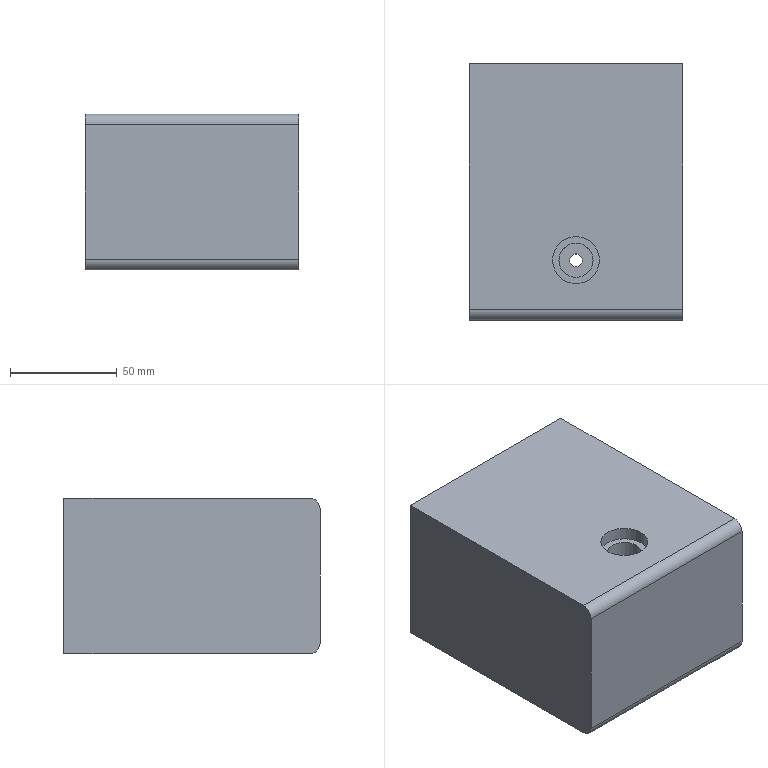Part | SolidWorks | features ICE 3, MoveFace 2, Extrusion 1, Fillet 1, HoleWzd 1 | 1 solid | 40 faces | box 100 x 120 x 73 mm | volume 861044 mm3 | cylinder 16 | cone 16 | plane 8 | commonest cylinder face diameters 8.5 x8 6 x2 10 x2 16 x2 22 x2
STEP:
#1=CARTESIAN_POINT('',(-8.,38.,6.5));
#2=VERTEX_POINT('',#1);
#3=CARTESIAN_POINT('',(8.,38.,6.5));
#4=VERTEX_POINT('',#3);
#5=CARTESIAN_POINT('',(0.,38.,6.5));
#6=DIRECTION('',(0.,0.,1.));
#7=DIRECTION('',(1.,0.,0.));
#8=AXIS2_PLACEMENT_3D('',#5,#6,#7);
#9=CIRCLE('',#8,8.);
#10=EDGE_CURVE('',#2,#4,#9,.T.);
#11=ORIENTED_EDGE('',*,*,#10,.F.);
#12=CARTESIAN_POINT('',(-8.,38.,30.5));
#13=VERTEX_POINT('',#12);
#14=CARTESIAN_POINT('',(-8.,38.,6.5));
#15=DIRECTION('',(0.,0.,1.));
#16=VECTOR('',#15,1000.);
#17=LINE('',#14,#16);
#18=EDGE_CURVE('',#2,#13,#17,.T.);
#19=ORIENTED_EDGE('',*,*,#18,.T.);
#20=CARTESIAN_POINT('',(8.,38.,30.5));
#21=VERTEX_POINT('',#20);
#22=CARTESIAN_POINT('',(0.,38.,30.5));
#23=DIRECTION('',(0.,0.,1.));
#24=DIRECTION('',(1.,0.,0.));
#25=AXIS2_PLACEMENT_3D('',#22,#23,#24);
#26=CIRCLE('',#25,8.);
#27=EDGE_CURVE('',#13,#21,#26,.T.);
#28=ORIENTED_EDGE('',*,*,#27,.T.);
#29=CARTESIAN_POINT('',(8.,38.,6.5));
#30=DIRECTION('',(0.,0.,1.));
#31=VECTOR('',#30,1000.);
#32=LINE('',#29,#31);
#33=EDGE_CURVE('',#4,#21,#32,.T.);
#34=ORIENTED_EDGE('',*,*,#33,.F.);
#35=EDGE_LOOP('',(#11,#19,#28,#34));
#36=FACE_OUTER_BOUND('',#35,.T.);
#37=CARTESIAN_POINT('',(0.,38.,6.5));
#38=DIRECTION('',(0.,0.,1.));
#39=DIRECTION('',(1.,0.,0.));
#40=AXIS2_PLACEMENT_3D('',#37,#38,#39);
#41=CYLINDRICAL_SURFACE('',#40,8.);
#42=ADVANCED_FACE('',(#36),#41,.F.);
#43=CARTESIAN_POINT('',(-11.,38.,30.5));
#44=VERTEX_POINT('',#43);
#45=CARTESIAN_POINT('',(11.,38.,30.5));
#46=VERTEX_POINT('',#45);
#47=CARTESIAN_POINT('',(0.,38.,30.5));
#48=DIRECTION('',(0.,0.,1.));
#49=DIRECTION('',(1.,0.,0.));
#50=AXIS2_PLACEMENT_3D('',#47,#48,#49);
#51=CIRCLE('',#50,11.);
#52=EDGE_CURVE('',#44,#46,#51,.T.);
#53=ORIENTED_EDGE('',*,*,#52,.F.);
#54=CARTESIAN_POINT('',(-11.,38.,36.5));
#55=VERTEX_POINT('',#54);
#56=CARTESIAN_POINT('',(-11.,38.,30.5));
#57=DIRECTION('',(0.,0.,1.));
#58=VECTOR('',#57,1000.);
#59=LINE('',#56,#58);
#60=EDGE_CURVE('',#44,#55,#59,.T.);
#61=ORIENTED_EDGE('',*,*,#60,.T.);
#62=CARTESIAN_POINT('',(11.,38.,36.5));
#63=VERTEX_POINT('',#62);
#64=CARTESIAN_POINT('',(0.,38.,36.5));
#65=DIRECTION('',(0.,0.,1.));
#66=DIRECTION('',(1.,0.,0.));
#67=AXIS2_PLACEMENT_3D('',#64,#65,#66);
#68=CIRCLE('',#67,11.);
#69=EDGE_CURVE('',#55,#63,#68,.T.);
#70=ORIENTED_EDGE('',*,*,#69,.T.);
#71=CARTESIAN_POINT('',(11.,38.,30.5));
#72=DIRECTION('',(0.,0.,1.));
#73=VECTOR('',#72,1000.);
#74=LINE('',#71,#73);
#75=EDGE_CURVE('',#46,#63,#74,.T.);
#76=ORIENTED_EDGE('',*,*,#75,.F.);
#77=EDGE_LOOP('',(#53,#61,#70,#76));
#78=FACE_OUTER_BOUND('',#77,.T.);
#79=CARTESIAN_POINT('',(0.,38.,30.5));
#80=DIRECTION('',(0.,0.,1.));
#81=DIRECTION('',(1.,0.,0.));
#82=AXIS2_PLACEMENT_3D('',#79,#80,#81);
#83=CYLINDRICAL_SURFACE('',#82,11.);
#84=ADVANCED_FACE('',(#78),#83,.F.);
#85=CARTESIAN_POINT('',(-40.,129.225,-30.75));
#86=VERTEX_POINT('',#85);
#87=CARTESIAN_POINT('',(-40.,129.225,-22.25));
#88=VERTEX_POINT('',#87);
#89=CARTESIAN_POINT('',(-40.,129.225,-26.5));
#90=DIRECTION('',(0.,1.,0.));
#91=DIRECTION('',(0.,0.,1.));
#92=AXIS2_PLACEMENT_3D('',#89,#90,#91);
#93=CIRCLE('',#92,4.25);
#94=EDGE_CURVE('',#86,#88,#93,.T.);
#95=ORIENTED_EDGE('',*,*,#94,.F.);
#96=CARTESIAN_POINT('',(-40.,130.,-31.525));
#97=VERTEX_POINT('',#96);
#98=CARTESIAN_POINT('',(-40.,130.,-31.525));
#99=DIRECTION('',(0.,0.7071,-0.7071));
#100=VECTOR('',#99,1000.);
#101=LINE('',#98,#100);
#102=EDGE_CURVE('',#86,#97,#101,.T.);
#103=ORIENTED_EDGE('',*,*,#102,.T.);
#104=CARTESIAN_POINT('',(-40.,130.,-21.475));
#105=VERTEX_POINT('',#104);
#106=CARTESIAN_POINT('',(-40.,130.,-26.5));
#107=DIRECTION('',(0.,1.,0.));
#108=DIRECTION('',(0.,0.,1.));
#109=AXIS2_PLACEMENT_3D('',#106,#107,#108);
#110=CIRCLE('',#109,5.025);
#111=EDGE_CURVE('',#97,#105,#110,.T.);
#112=ORIENTED_EDGE('',*,*,#111,.T.);
#113=CARTESIAN_POINT('',(-40.,130.,-21.475));
#114=DIRECTION('',(0.,0.7071,0.7071));
#115=VECTOR('',#114,1000.);
#116=LINE('',#113,#115);
#117=EDGE_CURVE('',#88,#105,#116,.T.);
#118=ORIENTED_EDGE('',*,*,#117,.F.);
#119=EDGE_LOOP('',(#95,#103,#112,#118));
#120=FACE_OUTER_BOUND('',#119,.T.);
#121=CARTESIAN_POINT('',(-40.,130.,-26.5));
#122=DIRECTION('',(0.,1.,0.));
#123=DIRECTION('',(0.,0.,1.));
#124=AXIS2_PLACEMENT_3D('',#121,#122,#123);
#125=CONICAL_SURFACE('',#124,5.025,0.7854);
#126=ADVANCED_FACE('',(#120),#125,.F.);
#127=CARTESIAN_POINT('',(-40.,106.5,-30.75));
#128=VERTEX_POINT('',#127);
#129=CARTESIAN_POINT('',(-40.,106.5,-22.25));
#130=VERTEX_POINT('',#129);
#131=CARTESIAN_POINT('',(-40.,106.5,-26.5));
#132=DIRECTION('',(0.,1.,0.));
#133=DIRECTION('',(0.,0.,1.));
#134=AXIS2_PLACEMENT_3D('',#131,#132,#133);
#135=CIRCLE('',#134,4.25);
#136=EDGE_CURVE('',#128,#130,#135,.T.);
#137=ORIENTED_EDGE('',*,*,#136,.F.);
#138=CARTESIAN_POINT('',(-40.,130.,-30.75));
#139=DIRECTION('',(0.,1.,0.));
#140=VECTOR('',#139,1000.);
#141=LINE('',#138,#140);
#142=EDGE_CURVE('',#128,#86,#141,.T.);
#143=ORIENTED_EDGE('',*,*,#142,.T.);
#144=ORIENTED_EDGE('',*,*,#94,.T.);
#145=CARTESIAN_POINT('',(-40.,130.,-22.25));
#146=DIRECTION('',(0.,1.,0.));
#147=VECTOR('',#146,1000.);
#148=LINE('',#145,#147);
#149=EDGE_CURVE('',#130,#88,#148,.T.);
#150=ORIENTED_EDGE('',*,*,#149,.F.);
#151=EDGE_LOOP('',(#137,#143,#144,#150));
#152=FACE_OUTER_BOUND('',#151,.T.);
#153=CARTESIAN_POINT('',(-40.,130.,-26.5));
#154=DIRECTION('',(0.,1.,0.));
#155=DIRECTION('',(0.,0.,1.));
#156=AXIS2_PLACEMENT_3D('',#153,#154,#155);
#157=CYLINDRICAL_SURFACE('',#156,4.25);
#158=ADVANCED_FACE('',(#152),#157,.F.);
#159=CARTESIAN_POINT('',(-40.,103.946,-26.5));
#160=VERTEX_POINT('',#159);
#161=CARTESIAN_POINT('',(-40.,106.5,-22.25));
#162=DIRECTION('',(0.,0.515,0.8572));
#163=VECTOR('',#162,1000.);
#164=LINE('',#161,#163);
#165=EDGE_CURVE('',#160,#130,#164,.T.);
#166=ORIENTED_EDGE('',*,*,#165,.F.);
#167=CARTESIAN_POINT('',(-40.,106.5,-30.75));
#168=DIRECTION('',(0.,0.515,-0.8572));
#169=VECTOR('',#168,1000.);
#170=LINE('',#167,#169);
#171=EDGE_CURVE('',#160,#128,#170,.T.);
#172=ORIENTED_EDGE('',*,*,#171,.T.);
#173=ORIENTED_EDGE('',*,*,#136,.T.);
#174=EDGE_LOOP('',(#166,#172,#173));
#175=FACE_OUTER_BOUND('',#174,.T.);
#176=CARTESIAN_POINT('',(-40.,106.5,-26.5));
#177=DIRECTION('',(0.,1.,0.));
#178=DIRECTION('',(0.,0.,1.));
#179=AXIS2_PLACEMENT_3D('',#176,#177,#178);
#180=CONICAL_SURFACE('',#179,4.25,1.03);
#181=ADVANCED_FACE('',(#175),#180,.F.);
#182=CARTESIAN_POINT('',(40.,129.225,-30.75));
#183=VERTEX_POINT('',#182);
#184=CARTESIAN_POINT('',(40.,129.225,-22.25));
#185=VERTEX_POINT('',#184);
#186=CARTESIAN_POINT('',(40.,129.225,-26.5));
#187=DIRECTION('',(0.,1.,0.));
#188=DIRECTION('',(0.,0.,1.));
#189=AXIS2_PLACEMENT_3D('',#186,#187,#188);
#190=CIRCLE('',#189,4.25);
#191=EDGE_CURVE('',#183,#185,#190,.T.);
#192=ORIENTED_EDGE('',*,*,#191,.F.);
#193=CARTESIAN_POINT('',(40.,130.,-31.525));
#194=VERTEX_POINT('',#193);
#195=CARTESIAN_POINT('',(40.,130.,-31.525));
#196=DIRECTION('',(0.,0.7071,-0.7071));
#197=VECTOR('',#196,1000.);
#198=LINE('',#195,#197);
#199=EDGE_CURVE('',#183,#194,#198,.T.);
#200=ORIENTED_EDGE('',*,*,#199,.T.);
#201=CARTESIAN_POINT('',(40.,130.,-21.475));
#202=VERTEX_POINT('',#201);
#203=CARTESIAN_POINT('',(40.,130.,-26.5));
#204=DIRECTION('',(0.,1.,0.));
#205=DIRECTION('',(0.,0.,1.));
#206=AXIS2_PLACEMENT_3D('',#203,#204,#205);
#207=CIRCLE('',#206,5.025);
#208=EDGE_CURVE('',#194,#202,#207,.T.);
#209=ORIENTED_EDGE('',*,*,#208,.T.);
#210=CARTESIAN_POINT('',(40.,130.,-21.475));
#211=DIRECTION('',(0.,0.7071,0.7071));
#212=VECTOR('',#211,1000.);
#213=LINE('',#210,#212);
#214=EDGE_CURVE('',#185,#202,#213,.T.);
#215=ORIENTED_EDGE('',*,*,#214,.F.);
#216=EDGE_LOOP('',(#192,#200,#209,#215));
#217=FACE_OUTER_BOUND('',#216,.T.);
#218=CARTESIAN_POINT('',(40.,130.,-26.5));
#219=DIRECTION('',(0.,1.,0.));
#220=DIRECTION('',(0.,0.,1.));
#221=AXIS2_PLACEMENT_3D('',#218,#219,#220);
#222=CONICAL_SURFACE('',#221,5.025,0.7854);
#223=ADVANCED_FACE('',(#217),#222,.F.);
#224=CARTESIAN_POINT('',(40.,106.5,-30.75));
#225=VERTEX_POINT('',#224);
#226=CARTESIAN_POINT('',(40.,106.5,-22.25));
#227=VERTEX_POINT('',#226);
#228=CARTESIAN_POINT('',(40.,106.5,-26.5));
#229=DIRECTION('',(0.,1.,0.));
#230=DIRECTION('',(0.,0.,1.));
#231=AXIS2_PLACEMENT_3D('',#228,#229,#230);
#232=CIRCLE('',#231,4.25);
#233=EDGE_CURVE('',#225,#227,#232,.T.);
#234=ORIENTED_EDGE('',*,*,#233,.F.);
#235=CARTESIAN_POINT('',(40.,130.,-30.75));
#236=DIRECTION('',(0.,1.,0.));
#237=VECTOR('',#236,1000.);
#238=LINE('',#235,#237);
#239=EDGE_CURVE('',#225,#183,#238,.T.);
#240=ORIENTED_EDGE('',*,*,#239,.T.);
#241=ORIENTED_EDGE('',*,*,#191,.T.);
#242=CARTESIAN_POINT('',(40.,130.,-22.25));
#243=DIRECTION('',(0.,1.,0.));
#244=VECTOR('',#243,1000.);
#245=LINE('',#242,#244);
#246=EDGE_CURVE('',#227,#185,#245,.T.);
#247=ORIENTED_EDGE('',*,*,#246,.F.);
#248=EDGE_LOOP('',(#234,#240,#241,#247));
#249=FACE_OUTER_BOUND('',#248,.T.);
#250=CARTESIAN_POINT('',(40.,130.,-26.5));
#251=DIRECTION('',(0.,1.,0.));
#252=DIRECTION('',(0.,0.,1.));
#253=AXIS2_PLACEMENT_3D('',#250,#251,#252);
#254=CYLINDRICAL_SURFACE('',#253,4.25);
#255=ADVANCED_FACE('',(#249),#254,.F.);
#256=CARTESIAN_POINT('',(40.,103.946,-26.5));
#257=VERTEX_POINT('',#256);
#258=CARTESIAN_POINT('',(40.,106.5,-22.25));
#259=DIRECTION('',(0.,0.515,0.8572));
#260=VECTOR('',#259,1000.);
#261=LINE('',#258,#260);
#262=EDGE_CURVE('',#257,#227,#261,.T.);
#263=ORIENTED_EDGE('',*,*,#262,.F.);
#264=CARTESIAN_POINT('',(40.,106.5,-30.75));
#265=DIRECTION('',(0.,0.515,-0.8572));
#266=VECTOR('',#265,1000.);
#267=LINE('',#264,#266);
#268=EDGE_CURVE('',#257,#225,#267,.T.);
#269=ORIENTED_EDGE('',*,*,#268,.T.);
#270=ORIENTED_EDGE('',*,*,#233,.T.);
#271=EDGE_LOOP('',(#263,#269,#270));
#272=FACE_OUTER_BOUND('',#271,.T.);
#273=CARTESIAN_POINT('',(40.,106.5,-26.5));
#274=DIRECTION('',(0.,1.,0.));
#275=DIRECTION('',(0.,0.,1.));
#276=AXIS2_PLACEMENT_3D('',#273,#274,#275);
#277=CONICAL_SURFACE('',#276,4.25,1.03);
#278=ADVANCED_FACE('',(#272),#277,.F.);
#279=CARTESIAN_POINT('',(40.,129.225,2.25));
#280=VERTEX_POINT('',#279);
#281=CARTESIAN_POINT('',(40.,129.225,10.75));
#282=VERTEX_POINT('',#281);
#283=CARTESIAN_POINT('',(40.,129.225,6.5));
#284=DIRECTION('',(0.,1.,0.));
#285=DIRECTION('',(0.,0.,1.));
#286=AXIS2_PLACEMENT_3D('',#283,#284,#285);
#287=CIRCLE('',#286,4.25);
#288=EDGE_CURVE('',#280,#282,#287,.T.);
#289=ORIENTED_EDGE('',*,*,#288,.F.);
#290=CARTESIAN_POINT('',(40.,130.,1.475));
#291=VERTEX_POINT('',#290);
#292=CARTESIAN_POINT('',(40.,130.,1.475));
#293=DIRECTION('',(0.,0.7071,-0.7071));
#294=VECTOR('',#293,1000.);
#295=LINE('',#292,#294);
#296=EDGE_CURVE('',#280,#291,#295,.T.);
#297=ORIENTED_EDGE('',*,*,#296,.T.);
#298=CARTESIAN_POINT('',(40.,130.,11.525));
#299=VERTEX_POINT('',#298);
#300=CARTESIAN_POINT('',(40.,130.,6.5));
#301=DIRECTION('',(0.,1.,0.));
#302=DIRECTION('',(0.,0.,1.));
#303=AXIS2_PLACEMENT_3D('',#300,#301,#302);
#304=CIRCLE('',#303,5.025);
#305=EDGE_CURVE('',#291,#299,#304,.T.);
#306=ORIENTED_EDGE('',*,*,#305,.T.);
#307=CARTESIAN_POINT('',(40.,130.,11.525));
#308=DIRECTION('',(0.,0.7071,0.7071));
#309=VECTOR('',#308,1000.);
#310=LINE('',#307,#309);
#311=EDGE_CURVE('',#282,#299,#310,.T.);
#312=ORIENTED_EDGE('',*,*,#311,.F.);
#313=EDGE_LOOP('',(#289,#297,#306,#312));
#314=FACE_OUTER_BOUND('',#313,.T.);
#315=CARTESIAN_POINT('',(40.,130.,6.5));
#316=DIRECTION('',(0.,1.,0.));
#317=DIRECTION('',(0.,0.,1.));
#318=AXIS2_PLACEMENT_3D('',#315,#316,#317);
#319=CONICAL_SURFACE('',#318,5.025,0.7854);
#320=ADVANCED_FACE('',(#314),#319,.F.);
#321=CARTESIAN_POINT('',(40.,106.5,2.25));
#322=VERTEX_POINT('',#321);
#323=CARTESIAN_POINT('',(40.,106.5,10.75));
#324=VERTEX_POINT('',#323);
#325=CARTESIAN_POINT('',(40.,106.5,6.5));
#326=DIRECTION('',(0.,1.,0.));
#327=DIRECTION('',(0.,0.,1.));
#328=AXIS2_PLACEMENT_3D('',#325,#326,#327);
#329=CIRCLE('',#328,4.25);
#330=EDGE_CURVE('',#322,#324,#329,.T.);
#331=ORIENTED_EDGE('',*,*,#330,.F.);
#332=CARTESIAN_POINT('',(40.,130.,2.25));
#333=DIRECTION('',(0.,1.,0.));
#334=VECTOR('',#333,1000.);
#335=LINE('',#332,#334);
#336=EDGE_CURVE('',#322,#280,#335,.T.);
#337=ORIENTED_EDGE('',*,*,#336,.T.);
#338=ORIENTED_EDGE('',*,*,#288,.T.);
#339=CARTESIAN_POINT('',(40.,130.,10.75));
#340=DIRECTION('',(0.,1.,0.));
#341=VECTOR('',#340,1000.);
#342=LINE('',#339,#341);
#343=EDGE_CURVE('',#324,#282,#342,.T.);
#344=ORIENTED_EDGE('',*,*,#343,.F.);
#345=EDGE_LOOP('',(#331,#337,#338,#344));
#346=FACE_OUTER_BOUND('',#345,.T.);
#347=CARTESIAN_POINT('',(40.,130.,6.5));
#348=DIRECTION('',(0.,1.,0.));
#349=DIRECTION('',(0.,0.,1.));
#350=AXIS2_PLACEMENT_3D('',#347,#348,#349);
#351=CYLINDRICAL_SURFACE('',#350,4.25);
#352=ADVANCED_FACE('',(#346),#351,.F.);
#353=CARTESIAN_POINT('',(40.,103.946,6.5));
#354=VERTEX_POINT('',#353);
#355=CARTESIAN_POINT('',(40.,106.5,10.75));
#356=DIRECTION('',(0.,0.515,0.8572));
#357=VECTOR('',#356,1000.);
#358=LINE('',#355,#357);
#359=EDGE_CURVE('',#354,#324,#358,.T.);
#360=ORIENTED_EDGE('',*,*,#359,.F.);
#361=CARTESIAN_POINT('',(40.,106.5,2.25));
#362=DIRECTION('',(0.,0.515,-0.8572));
#363=VECTOR('',#362,1000.);
#364=LINE('',#361,#363);
#365=EDGE_CURVE('',#354,#322,#364,.T.);
#366=ORIENTED_EDGE('',*,*,#365,.T.);
#367=ORIENTED_EDGE('',*,*,#330,.T.);
#368=EDGE_LOOP('',(#360,#366,#367));
#369=FACE_OUTER_BOUND('',#368,.T.);
#370=CARTESIAN_POINT('',(40.,106.5,6.5));
#371=DIRECTION('',(0.,1.,0.));
#372=DIRECTION('',(0.,0.,1.));
#373=AXIS2_PLACEMENT_3D('',#370,#371,#372);
#374=CONICAL_SURFACE('',#373,4.25,1.03);
#375=ADVANCED_FACE('',(#369),#374,.F.);
#376=CARTESIAN_POINT('',(-40.,129.225,2.25));
#377=VERTEX_POINT('',#376);
#378=CARTESIAN_POINT('',(-40.,129.225,10.75));
#379=VERTEX_POINT('',#378);
#380=CARTESIAN_POINT('',(-40.,129.225,6.5));
#381=DIRECTION('',(0.,1.,0.));
#382=DIRECTION('',(0.,0.,1.));
#383=AXIS2_PLACEMENT_3D('',#380,#381,#382);
#384=CIRCLE('',#383,4.25);
#385=EDGE_CURVE('',#377,#379,#384,.T.);
#386=ORIENTED_EDGE('',*,*,#385,.F.);
#387=CARTESIAN_POINT('',(-40.,130.,1.475));
#388=VERTEX_POINT('',#387);
#389=CARTESIAN_POINT('',(-40.,130.,1.475));
#390=DIRECTION('',(0.,0.7071,-0.7071));
#391=VECTOR('',#390,1000.);
#392=LINE('',#389,#391);
#393=EDGE_CURVE('',#377,#388,#392,.T.);
#394=ORIENTED_EDGE('',*,*,#393,.T.);
#395=CARTESIAN_POINT('',(-40.,130.,11.525));
#396=VERTEX_POINT('',#395);
#397=CARTESIAN_POINT('',(-40.,130.,6.5));
#398=DIRECTION('',(0.,1.,0.));
#399=DIRECTION('',(0.,0.,1.));
#400=AXIS2_PLACEMENT_3D('',#397,#398,#399);
#401=CIRCLE('',#400,5.025);
#402=EDGE_CURVE('',#388,#396,#401,.T.);
#403=ORIENTED_EDGE('',*,*,#402,.T.);
#404=CARTESIAN_POINT('',(-40.,130.,11.525));
#405=DIRECTION('',(0.,0.7071,0.7071));
#406=VECTOR('',#405,1000.);
#407=LINE('',#404,#406);
#408=EDGE_CURVE('',#379,#396,#407,.T.);
#409=ORIENTED_EDGE('',*,*,#408,.F.);
#410=EDGE_LOOP('',(#386,#394,#403,#409));
#411=FACE_OUTER_BOUND('',#410,.T.);
#412=CARTESIAN_POINT('',(-40.,130.,6.5));
#413=DIRECTION('',(0.,1.,0.));
#414=DIRECTION('',(0.,0.,1.));
#415=AXIS2_PLACEMENT_3D('',#412,#413,#414);
#416=CONICAL_SURFACE('',#415,5.025,0.7854);
#417=ADVANCED_FACE('',(#411),#416,.F.);
#418=CARTESIAN_POINT('',(-40.,106.5,2.25));
#419=VERTEX_POINT('',#418);
#420=CARTESIAN_POINT('',(-40.,106.5,10.75));
#421=VERTEX_POINT('',#420);
#422=CARTESIAN_POINT('',(-40.,106.5,6.5));
#423=DIRECTION('',(0.,1.,0.));
#424=DIRECTION('',(0.,0.,1.));
#425=AXIS2_PLACEMENT_3D('',#422,#423,#424);
#426=CIRCLE('',#425,4.25);
#427=EDGE_CURVE('',#419,#421,#426,.T.);
#428=ORIENTED_EDGE('',*,*,#427,.F.);
#429=CARTESIAN_POINT('',(-40.,130.,2.25));
#430=DIRECTION('',(0.,1.,0.));
#431=VECTOR('',#430,1000.);
#432=LINE('',#429,#431);
#433=EDGE_CURVE('',#419,#377,#432,.T.);
#434=ORIENTED_EDGE('',*,*,#433,.T.);
#435=ORIENTED_EDGE('',*,*,#385,.T.);
#436=CARTESIAN_POINT('',(-40.,130.,10.75));
#437=DIRECTION('',(0.,1.,0.));
#438=VECTOR('',#437,1000.);
#439=LINE('',#436,#438);
#440=EDGE_CURVE('',#421,#379,#439,.T.);
#441=ORIENTED_EDGE('',*,*,#440,.F.);
#442=EDGE_LOOP('',(#428,#434,#435,#441));
#443=FACE_OUTER_BOUND('',#442,.T.);
#444=CARTESIAN_POINT('',(-40.,130.,6.5));
#445=DIRECTION('',(0.,1.,0.));
#446=DIRECTION('',(0.,0.,1.));
#447=AXIS2_PLACEMENT_3D('',#444,#445,#446);
#448=CYLINDRICAL_SURFACE('',#447,4.25);
#449=ADVANCED_FACE('',(#443),#448,.F.);
#450=CARTESIAN_POINT('',(-40.,103.946,6.5));
#451=VERTEX_POINT('',#450);
#452=CARTESIAN_POINT('',(-40.,106.5,10.75));
#453=DIRECTION('',(0.,0.515,0.8572));
#454=VECTOR('',#453,1000.);
#455=LINE('',#452,#454);
#456=EDGE_CURVE('',#451,#421,#455,.T.);
#457=ORIENTED_EDGE('',*,*,#456,.F.);
#458=CARTESIAN_POINT('',(-40.,106.5,2.25));
#459=DIRECTION('',(0.,0.515,-0.8572));
#460=VECTOR('',#459,1000.);
#461=LINE('',#458,#460);
#462=EDGE_CURVE('',#451,#419,#461,.T.);
#463=ORIENTED_EDGE('',*,*,#462,.T.);
#464=ORIENTED_EDGE('',*,*,#427,.T.);
#465=EDGE_LOOP('',(#457,#463,#464));
#466=FACE_OUTER_BOUND('',#465,.T.);
#467=CARTESIAN_POINT('',(-40.,106.5,6.5));
#468=DIRECTION('',(0.,1.,0.));
#469=DIRECTION('',(0.,0.,1.));
#470=AXIS2_PLACEMENT_3D('',#467,#468,#469);
#471=CONICAL_SURFACE('',#470,4.25,1.03);
#472=ADVANCED_FACE('',(#466),#471,.F.);
#473=CARTESIAN_POINT('',(3.,38.,6.5));
#474=VERTEX_POINT('',#473);
#475=CARTESIAN_POINT('',(-3.,38.,6.5));
#476=VERTEX_POINT('',#475);
#477=CARTESIAN_POINT('',(0.,38.,6.5));
#478=DIRECTION('',(0.,0.,-1.));
#479=DIRECTION('',(1.,0.,0.));
#480=AXIS2_PLACEMENT_3D('',#477,#478,#479);
#481=CIRCLE('',#480,3.);
#482=EDGE_CURVE('',#474,#476,#481,.T.);
#483=ORIENTED_EDGE('',*,*,#482,.F.);
#484=CARTESIAN_POINT('',(3.,38.,-36.5));
#485=VERTEX_POINT('',#484);
#486=CARTESIAN_POINT('',(3.,38.,93.5));
#487=DIRECTION('',(0.,0.,-1.));
#488=VECTOR('',#487,1000.);
#489=LINE('',#486,#488);
#490=EDGE_CURVE('',#474,#485,#489,.T.);
#491=ORIENTED_EDGE('',*,*,#490,.T.);
#492=CARTESIAN_POINT('',(-3.,38.,-36.5));
#493=VERTEX_POINT('',#492);
#494=CARTESIAN_POINT('',(0.,38.,-36.5));
#495=DIRECTION('',(0.,0.,-1.));
#496=DIRECTION('',(-1.,0.,0.));
#497=AXIS2_PLACEMENT_3D('',#494,#495,#496);
#498=CIRCLE('',#497,3.);
#499=EDGE_CURVE('',#485,#493,#498,.T.);
#500=ORIENTED_EDGE('',*,*,#499,.T.);
#501=CARTESIAN_POINT('',(-3.,38.,93.5));
#502=DIRECTION('',(0.,0.,-1.));
#503=VECTOR('',#502,1000.);
#504=LINE('',#501,#503);
#505=EDGE_CURVE('',#476,#493,#504,.T.);
#506=ORIENTED_EDGE('',*,*,#505,.F.);
#507=EDGE_LOOP('',(#483,#491,#500,#506));
#508=FACE_OUTER_BOUND('',#507,.T.);
#509=CARTESIAN_POINT('',(0.,38.,93.5));
#510=DIRECTION('',(0.,0.,-1.));
#511=DIRECTION('',(-1.,0.,0.));
#512=AXIS2_PLACEMENT_3D('',#509,#510,#511);
#513=CYLINDRICAL_SURFACE('',#512,3.);
#514=ADVANCED_FACE('',(#508),#513,.F.);
#515=ORIENTED_EDGE('',*,*,#490,.F.);
#516=CARTESIAN_POINT('',(0.,38.,6.5));
#517=DIRECTION('',(0.,0.,-1.));
#518=DIRECTION('',(1.,0.,0.));
#519=AXIS2_PLACEMENT_3D('',#516,#517,#518);
#520=CIRCLE('',#519,3.);
#521=EDGE_CURVE('',#476,#474,#520,.T.);
#522=ORIENTED_EDGE('',*,*,#521,.F.);
#523=ORIENTED_EDGE('',*,*,#505,.T.);
#524=CARTESIAN_POINT('',(0.,38.,-36.5));
#525=DIRECTION('',(0.,0.,-1.));
#526=DIRECTION('',(-1.,0.,0.));
#527=AXIS2_PLACEMENT_3D('',#524,#525,#526);
#528=CIRCLE('',#527,3.);
#529=EDGE_CURVE('',#493,#485,#528,.T.);
#530=ORIENTED_EDGE('',*,*,#529,.T.);
#531=EDGE_LOOP('',(#515,#522,#523,#530));
#532=FACE_OUTER_BOUND('',#531,.T.);
#533=CARTESIAN_POINT('',(0.,38.,93.5));
#534=DIRECTION('',(0.,0.,-1.));
#535=DIRECTION('',(-1.,0.,0.));
#536=AXIS2_PLACEMENT_3D('',#533,#534,#535);
#537=CYLINDRICAL_SURFACE('',#536,3.);
#538=ADVANCED_FACE('',(#532),#537,.F.);
#539=CARTESIAN_POINT('',(50.,10.,31.5));
#540=VERTEX_POINT('',#539);
#541=CARTESIAN_POINT('',(50.,10.,-31.5));
#542=VERTEX_POINT('',#541);
#543=CARTESIAN_POINT('',(50.,10.,36.5));
#544=DIRECTION('',(0.,0.,-1.));
#545=VECTOR('',#544,1000.);
#546=LINE('',#543,#545);
#547=EDGE_CURVE('',#540,#542,#546,.T.);
#548=ORIENTED_EDGE('',*,*,#547,.T.);
#549=CARTESIAN_POINT('',(50.,15.,-36.5));
#550=VERTEX_POINT('',#549);
#551=CARTESIAN_POINT('',(50.,15.,-31.5));
#552=DIRECTION('',(1.,0.,0.));
#553=DIRECTION('',(0.,0.,1.));
#554=AXIS2_PLACEMENT_3D('',#551,#552,#553);
#555=CIRCLE('',#554,5.);
#556=EDGE_CURVE('',#542,#550,#555,.T.);
#557=ORIENTED_EDGE('',*,*,#556,.T.);
#558=CARTESIAN_POINT('',(50.,130.,-36.5));
#559=VERTEX_POINT('',#558);
#560=CARTESIAN_POINT('',(50.,130.,-36.5));
#561=DIRECTION('',(0.,-1.,0.));
#562=VECTOR('',#561,1000.);
#563=LINE('',#560,#562);
#564=EDGE_CURVE('',#559,#550,#563,.T.);
#565=ORIENTED_EDGE('',*,*,#564,.F.);
#566=CARTESIAN_POINT('',(50.,130.,36.5));
#567=VERTEX_POINT('',#566);
#568=CARTESIAN_POINT('',(50.,130.,36.5));
#569=DIRECTION('',(0.,0.,-1.));
#570=VECTOR('',#569,1000.);
#571=LINE('',#568,#570);
#572=EDGE_CURVE('',#567,#559,#571,.T.);
#573=ORIENTED_EDGE('',*,*,#572,.F.);
#574=CARTESIAN_POINT('',(50.,15.,36.5));
#575=VERTEX_POINT('',#574);
#576=CARTESIAN_POINT('',(50.,130.,36.5));
#577=DIRECTION('',(0.,-1.,0.));
#578=VECTOR('',#577,1000.);
#579=LINE('',#576,#578);
#580=EDGE_CURVE('',#567,#575,#579,.T.);
#581=ORIENTED_EDGE('',*,*,#580,.T.);
#582=CARTESIAN_POINT('',(50.,15.,31.5));
#583=DIRECTION('',(1.,0.,0.));
#584=DIRECTION('',(0.,0.,1.));
#585=AXIS2_PLACEMENT_3D('',#582,#583,#584);
#586=CIRCLE('',#585,5.);
#587=EDGE_CURVE('',#575,#540,#586,.T.);
#588=ORIENTED_EDGE('',*,*,#587,.T.);
#589=EDGE_LOOP('',(#548,#557,#565,#573,#581,#588));
#590=FACE_OUTER_BOUND('',#589,.T.);
#591=CARTESIAN_POINT('',(50.,130.,36.5));
#592=DIRECTION('',(-1.,0.,0.));
#593=DIRECTION('',(0.,0.,1.));
#594=AXIS2_PLACEMENT_3D('',#591,#592,#593);
#595=PLANE('',#594);
#596=ADVANCED_FACE('',(#590),#595,.F.);
#597=ORIENTED_EDGE('',*,*,#529,.F.);
#598=ORIENTED_EDGE('',*,*,#499,.F.);
#599=EDGE_LOOP('',(#597,#598));
#600=FACE_BOUND('',#599,.T.);
#601=ORIENTED_EDGE('',*,*,#564,.T.);
#602=CARTESIAN_POINT('',(-50.,15.,-36.5));
#603=VERTEX_POINT('',#602);
#604=CARTESIAN_POINT('',(-50.,15.,-36.5));
#605=DIRECTION('',(-1.,0.,0.));
#606=VECTOR('',#605,1000.);
#607=LINE('',#604,#606);
#608=EDGE_CURVE('',#550,#603,#607,.T.);
#609=ORIENTED_EDGE('',*,*,#608,.T.);
#610=CARTESIAN_POINT('',(-50.,130.,-36.5));
#611=VERTEX_POINT('',#610);
#612=CARTESIAN_POINT('',(-50.,130.,-36.5));
#613=DIRECTION('',(0.,-1.,0.));
#614=VECTOR('',#613,1000.);
#615=LINE('',#612,#614);
#616=EDGE_CURVE('',#611,#603,#615,.T.);
#617=ORIENTED_EDGE('',*,*,#616,.F.);
#618=CARTESIAN_POINT('',(-50.,130.,-36.5));
#619=DIRECTION('',(-1.,0.,0.));
#620=VECTOR('',#619,1000.);
#621=LINE('',#618,#620);
#622=EDGE_CURVE('',#559,#611,#621,.T.);
#623=ORIENTED_EDGE('',*,*,#622,.F.);
#624=EDGE_LOOP('',(#601,#609,#617,#623));
#625=FACE_OUTER_BOUND('',#624,.T.);
#626=CARTESIAN_POINT('',(-50.,130.,-36.5));
#627=DIRECTION('',(0.,0.,1.));
#628=DIRECTION('',(1.,0.,0.));
#629=AXIS2_PLACEMENT_3D('',#626,#627,#628);
#630=PLANE('',#629);
#631=ADVANCED_FACE('',(#600,#625),#630,.F.);
#632=ORIENTED_EDGE('',*,*,#616,.T.);
#633=CARTESIAN_POINT('',(-50.,10.,-31.5));
#634=VERTEX_POINT('',#633);
#635=CARTESIAN_POINT('',(-50.,15.,-31.5));
#636=DIRECTION('',(-1.,0.,0.));
#637=DIRECTION('',(0.,0.,-1.));
#638=AXIS2_PLACEMENT_3D('',#635,#636,#637);
#639=CIRCLE('',#638,5.);
#640=EDGE_CURVE('',#603,#634,#639,.T.);
#641=ORIENTED_EDGE('',*,*,#640,.T.);
#642=CARTESIAN_POINT('',(-50.,10.,31.5));
#643=VERTEX_POINT('',#642);
#644=CARTESIAN_POINT('',(-50.,10.,36.5));
#645=DIRECTION('',(0.,0.,1.));
#646=VECTOR('',#645,1000.);
#647=LINE('',#644,#646);
#648=EDGE_CURVE('',#634,#643,#647,.T.);
#649=ORIENTED_EDGE('',*,*,#648,.T.);
#650=CARTESIAN_POINT('',(-50.,15.,36.5));
#651=VERTEX_POINT('',#650);
#652=CARTESIAN_POINT('',(-50.,15.,31.5));
#653=DIRECTION('',(-1.,0.,0.));
#654=DIRECTION('',(0.,0.,-1.));
#655=AXIS2_PLACEMENT_3D('',#652,#653,#654);
#656=CIRCLE('',#655,5.);
#657=EDGE_CURVE('',#643,#651,#656,.T.);
#658=ORIENTED_EDGE('',*,*,#657,.T.);
#659=CARTESIAN_POINT('',(-50.,130.,36.5));
#660=VERTEX_POINT('',#659);
#661=CARTESIAN_POINT('',(-50.,130.,36.5));
#662=DIRECTION('',(0.,-1.,0.));
#663=VECTOR('',#662,1000.);
#664=LINE('',#661,#663);
#665=EDGE_CURVE('',#660,#651,#664,.T.);
#666=ORIENTED_EDGE('',*,*,#665,.F.);
#667=CARTESIAN_POINT('',(-50.,130.,36.5));
#668=DIRECTION('',(0.,0.,1.));
#669=VECTOR('',#668,1000.);
#670=LINE('',#667,#669);
#671=EDGE_CURVE('',#611,#660,#670,.T.);
#672=ORIENTED_EDGE('',*,*,#671,.F.);
#673=EDGE_LOOP('',(#632,#641,#649,#658,#666,#672));
#674=FACE_OUTER_BOUND('',#673,.T.);
#675=CARTESIAN_POINT('',(-50.,130.,36.5));
#676=DIRECTION('',(1.,0.,0.));
#677=DIRECTION('',(0.,0.,-1.));
#678=AXIS2_PLACEMENT_3D('',#675,#676,#677);
#679=PLANE('',#678);
#680=ADVANCED_FACE('',(#674),#679,.F.);
#681=CARTESIAN_POINT('',(0.,38.,36.5));
#682=DIRECTION('',(0.,0.,1.));
#683=DIRECTION('',(1.,0.,0.));
#684=AXIS2_PLACEMENT_3D('',#681,#682,#683);
#685=CIRCLE('',#684,11.);
#686=EDGE_CURVE('',#63,#55,#685,.T.);
#687=ORIENTED_EDGE('',*,*,#686,.F.);
#688=ORIENTED_EDGE('',*,*,#69,.F.);
#689=EDGE_LOOP('',(#687,#688));
#690=FACE_BOUND('',#689,.T.);
#691=ORIENTED_EDGE('',*,*,#665,.T.);
#692=CARTESIAN_POINT('',(50.,15.,36.5));
#693=DIRECTION('',(1.,0.,0.));
#694=VECTOR('',#693,1000.);
#695=LINE('',#692,#694);
#696=EDGE_CURVE('',#651,#575,#695,.T.);
#697=ORIENTED_EDGE('',*,*,#696,.T.);
#698=ORIENTED_EDGE('',*,*,#580,.F.);
#699=CARTESIAN_POINT('',(-50.,130.,36.5));
#700=DIRECTION('',(1.,0.,0.));
#701=VECTOR('',#700,1000.);
#702=LINE('',#699,#701);
#703=EDGE_CURVE('',#660,#567,#702,.T.);
#704=ORIENTED_EDGE('',*,*,#703,.F.);
#705=EDGE_LOOP('',(#691,#697,#698,#704));
#706=FACE_OUTER_BOUND('',#705,.T.);
#707=CARTESIAN_POINT('',(-50.,130.,36.5));
#708=DIRECTION('',(0.,0.,-1.));
#709=DIRECTION('',(-1.,0.,0.));
#710=AXIS2_PLACEMENT_3D('',#707,#708,#709);
#711=PLANE('',#710);
#712=ADVANCED_FACE('',(#690,#706),#711,.F.);
#713=CARTESIAN_POINT('',(-40.,130.,-26.5));
#714=DIRECTION('',(0.,1.,0.));
#715=DIRECTION('',(0.,0.,1.));
#716=AXIS2_PLACEMENT_3D('',#713,#714,#715);
#717=CIRCLE('',#716,5.025);
#718=EDGE_CURVE('',#105,#97,#717,.T.);
#719=ORIENTED_EDGE('',*,*,#718,.F.);
#720=ORIENTED_EDGE('',*,*,#111,.F.);
#721=EDGE_LOOP('',(#719,#720));
#722=FACE_BOUND('',#721,.T.);
#723=CARTESIAN_POINT('',(40.,130.,-26.5));
#724=DIRECTION('',(0.,1.,0.));
#725=DIRECTION('',(0.,0.,1.));
#726=AXIS2_PLACEMENT_3D('',#723,#724,#725);
#727=CIRCLE('',#726,5.025);
#728=EDGE_CURVE('',#202,#194,#727,.T.);
#729=ORIENTED_EDGE('',*,*,#728,.F.);
#730=ORIENTED_EDGE('',*,*,#208,.F.);
#731=EDGE_LOOP('',(#729,#730));
#732=FACE_BOUND('',#731,.T.);
#733=CARTESIAN_POINT('',(40.,130.,6.5));
#734=DIRECTION('',(0.,1.,0.));
#735=DIRECTION('',(0.,0.,1.));
#736=AXIS2_PLACEMENT_3D('',#733,#734,#735);
#737=CIRCLE('',#736,5.025);
#738=EDGE_CURVE('',#299,#291,#737,.T.);
#739=ORIENTED_EDGE('',*,*,#738,.F.);
#740=ORIENTED_EDGE('',*,*,#305,.F.);
#741=EDGE_LOOP('',(#739,#740));
#742=FACE_BOUND('',#741,.T.);
#743=CARTESIAN_POINT('',(-40.,130.,6.5));
#744=DIRECTION('',(0.,1.,0.));
#745=DIRECTION('',(0.,0.,1.));
#746=AXIS2_PLACEMENT_3D('',#743,#744,#745);
#747=CIRCLE('',#746,5.025);
#748=EDGE_CURVE('',#396,#388,#747,.T.);
#749=ORIENTED_EDGE('',*,*,#748,.F.);
#750=ORIENTED_EDGE('',*,*,#402,.F.);
#751=EDGE_LOOP('',(#749,#750));
#752=FACE_BOUND('',#751,.T.);
#753=ORIENTED_EDGE('',*,*,#572,.T.);
#754=ORIENTED_EDGE('',*,*,#622,.T.);
#755=ORIENTED_EDGE('',*,*,#671,.T.);
#756=ORIENTED_EDGE('',*,*,#703,.T.);
#757=EDGE_LOOP('',(#753,#754,#755,#756));
#758=FACE_OUTER_BOUND('',#757,.T.);
#759=CARTESIAN_POINT('',(0.,130.,0.));
#760=DIRECTION('',(0.,-1.,0.));
#761=DIRECTION('',(0.,0.,-1.));
#762=AXIS2_PLACEMENT_3D('',#759,#760,#761);
#763=PLANE('',#762);
#764=ADVANCED_FACE('',(#722,#732,#742,#752,#758),#763,.F.);
#765=ORIENTED_EDGE('',*,*,#648,.F.);
#766=CARTESIAN_POINT('',(50.,10.,-31.5));
#767=DIRECTION('',(1.,0.,0.));
#768=VECTOR('',#767,1000.);
#769=LINE('',#766,#768);
#770=EDGE_CURVE('',#634,#542,#769,.T.);
#771=ORIENTED_EDGE('',*,*,#770,.T.);
#772=ORIENTED_EDGE('',*,*,#547,.F.);
#773=CARTESIAN_POINT('',(-50.,10.,31.5));
#774=DIRECTION('',(-1.,0.,0.));
#775=VECTOR('',#774,1000.);
#776=LINE('',#773,#775);
#777=EDGE_CURVE('',#540,#643,#776,.T.);
#778=ORIENTED_EDGE('',*,*,#777,.T.);
#779=EDGE_LOOP('',(#765,#771,#772,#778));
#780=FACE_OUTER_BOUND('',#779,.T.);
#781=CARTESIAN_POINT('',(0.,10.,0.));
#782=DIRECTION('',(0.,-1.,0.));
#783=DIRECTION('',(0.,0.,-1.));
#784=AXIS2_PLACEMENT_3D('',#781,#782,#783);
#785=PLANE('',#784);
#786=ADVANCED_FACE('',(#780),#785,.T.);
#787=ORIENTED_EDGE('',*,*,#462,.F.);
#788=ORIENTED_EDGE('',*,*,#456,.T.);
#789=CARTESIAN_POINT('',(-40.,106.5,6.5));
#790=DIRECTION('',(0.,1.,0.));
#791=DIRECTION('',(0.,0.,1.));
#792=AXIS2_PLACEMENT_3D('',#789,#790,#791);
#793=CIRCLE('',#792,4.25);
#794=EDGE_CURVE('',#421,#419,#793,.T.);
#795=ORIENTED_EDGE('',*,*,#794,.T.);
#796=EDGE_LOOP('',(#787,#788,#795));
#797=FACE_OUTER_BOUND('',#796,.T.);
#798=CARTESIAN_POINT('',(-40.,106.5,6.5));
#799=DIRECTION('',(0.,1.,0.));
#800=DIRECTION('',(0.,0.,1.));
#801=AXIS2_PLACEMENT_3D('',#798,#799,#800);
#802=CONICAL_SURFACE('',#801,4.25,1.03);
#803=ADVANCED_FACE('',(#797),#802,.F.);
#804=ORIENTED_EDGE('',*,*,#433,.F.);
#805=ORIENTED_EDGE('',*,*,#794,.F.);
#806=ORIENTED_EDGE('',*,*,#440,.T.);
#807=CARTESIAN_POINT('',(-40.,129.225,6.5));
#808=DIRECTION('',(0.,1.,0.));
#809=DIRECTION('',(0.,0.,1.));
#810=AXIS2_PLACEMENT_3D('',#807,#808,#809);
#811=CIRCLE('',#810,4.25);
#812=EDGE_CURVE('',#379,#377,#811,.T.);
#813=ORIENTED_EDGE('',*,*,#812,.T.);
#814=EDGE_LOOP('',(#804,#805,#806,#813));
#815=FACE_OUTER_BOUND('',#814,.T.);
#816=CARTESIAN_POINT('',(-40.,130.,6.5));
#817=DIRECTION('',(0.,1.,0.));
#818=DIRECTION('',(0.,0.,1.));
#819=AXIS2_PLACEMENT_3D('',#816,#817,#818);
#820=CYLINDRICAL_SURFACE('',#819,4.25);
#821=ADVANCED_FACE('',(#815),#820,.F.);
#822=ORIENTED_EDGE('',*,*,#393,.F.);
#823=ORIENTED_EDGE('',*,*,#812,.F.);
#824=ORIENTED_EDGE('',*,*,#408,.T.);
#825=ORIENTED_EDGE('',*,*,#748,.T.);
#826=EDGE_LOOP('',(#822,#823,#824,#825));
#827=FACE_OUTER_BOUND('',#826,.T.);
#828=CARTESIAN_POINT('',(-40.,130.,6.5));
#829=DIRECTION('',(0.,1.,0.));
#830=DIRECTION('',(0.,0.,1.));
#831=AXIS2_PLACEMENT_3D('',#828,#829,#830);
#832=CONICAL_SURFACE('',#831,5.025,0.7854);
#833=ADVANCED_FACE('',(#827),#832,.F.);
#834=ORIENTED_EDGE('',*,*,#365,.F.);
#835=ORIENTED_EDGE('',*,*,#359,.T.);
#836=CARTESIAN_POINT('',(40.,106.5,6.5));
#837=DIRECTION('',(0.,1.,0.));
#838=DIRECTION('',(0.,0.,1.));
#839=AXIS2_PLACEMENT_3D('',#836,#837,#838);
#840=CIRCLE('',#839,4.25);
#841=EDGE_CURVE('',#324,#322,#840,.T.);
#842=ORIENTED_EDGE('',*,*,#841,.T.);
#843=EDGE_LOOP('',(#834,#835,#842));
#844=FACE_OUTER_BOUND('',#843,.T.);
#845=CARTESIAN_POINT('',(40.,106.5,6.5));
#846=DIRECTION('',(0.,1.,0.));
#847=DIRECTION('',(0.,0.,1.));
#848=AXIS2_PLACEMENT_3D('',#845,#846,#847);
#849=CONICAL_SURFACE('',#848,4.25,1.03);
#850=ADVANCED_FACE('',(#844),#849,.F.);
#851=ORIENTED_EDGE('',*,*,#336,.F.);
#852=ORIENTED_EDGE('',*,*,#841,.F.);
#853=ORIENTED_EDGE('',*,*,#343,.T.);
#854=CARTESIAN_POINT('',(40.,129.225,6.5));
#855=DIRECTION('',(0.,1.,0.));
#856=DIRECTION('',(0.,0.,1.));
#857=AXIS2_PLACEMENT_3D('',#854,#855,#856);
#858=CIRCLE('',#857,4.25);
#859=EDGE_CURVE('',#282,#280,#858,.T.);
#860=ORIENTED_EDGE('',*,*,#859,.T.);
#861=EDGE_LOOP('',(#851,#852,#853,#860));
#862=FACE_OUTER_BOUND('',#861,.T.);
#863=CARTESIAN_POINT('',(40.,130.,6.5));
#864=DIRECTION('',(0.,1.,0.));
#865=DIRECTION('',(0.,0.,1.));
#866=AXIS2_PLACEMENT_3D('',#863,#864,#865);
#867=CYLINDRICAL_SURFACE('',#866,4.25);
#868=ADVANCED_FACE('',(#862),#867,.F.);
#869=ORIENTED_EDGE('',*,*,#296,.F.);
#870=ORIENTED_EDGE('',*,*,#859,.F.);
#871=ORIENTED_EDGE('',*,*,#311,.T.);
#872=ORIENTED_EDGE('',*,*,#738,.T.);
#873=EDGE_LOOP('',(#869,#870,#871,#872));
#874=FACE_OUTER_BOUND('',#873,.T.);
#875=CARTESIAN_POINT('',(40.,130.,6.5));
#876=DIRECTION('',(0.,1.,0.));
#877=DIRECTION('',(0.,0.,1.));
#878=AXIS2_PLACEMENT_3D('',#875,#876,#877);
#879=CONICAL_SURFACE('',#878,5.025,0.7854);
#880=ADVANCED_FACE('',(#874),#879,.F.);
#881=ORIENTED_EDGE('',*,*,#268,.F.);
#882=ORIENTED_EDGE('',*,*,#262,.T.);
#883=CARTESIAN_POINT('',(40.,106.5,-26.5));
#884=DIRECTION('',(0.,1.,0.));
#885=DIRECTION('',(0.,0.,1.));
#886=AXIS2_PLACEMENT_3D('',#883,#884,#885);
#887=CIRCLE('',#886,4.25);
#888=EDGE_CURVE('',#227,#225,#887,.T.);
#889=ORIENTED_EDGE('',*,*,#888,.T.);
#890=EDGE_LOOP('',(#881,#882,#889));
#891=FACE_OUTER_BOUND('',#890,.T.);
#892=CARTESIAN_POINT('',(40.,106.5,-26.5));
#893=DIRECTION('',(0.,1.,0.));
#894=DIRECTION('',(0.,0.,1.));
#895=AXIS2_PLACEMENT_3D('',#892,#893,#894);
#896=CONICAL_SURFACE('',#895,4.25,1.03);
#897=ADVANCED_FACE('',(#891),#896,.F.);
#898=ORIENTED_EDGE('',*,*,#239,.F.);
#899=ORIENTED_EDGE('',*,*,#888,.F.);
#900=ORIENTED_EDGE('',*,*,#246,.T.);
#901=CARTESIAN_POINT('',(40.,129.225,-26.5));
#902=DIRECTION('',(0.,1.,0.));
#903=DIRECTION('',(0.,0.,1.));
#904=AXIS2_PLACEMENT_3D('',#901,#902,#903);
#905=CIRCLE('',#904,4.25);
#906=EDGE_CURVE('',#185,#183,#905,.T.);
#907=ORIENTED_EDGE('',*,*,#906,.T.);
#908=EDGE_LOOP('',(#898,#899,#900,#907));
#909=FACE_OUTER_BOUND('',#908,.T.);
#910=CARTESIAN_POINT('',(40.,130.,-26.5));
#911=DIRECTION('',(0.,1.,0.));
#912=DIRECTION('',(0.,0.,1.));
#913=AXIS2_PLACEMENT_3D('',#910,#911,#912);
#914=CYLINDRICAL_SURFACE('',#913,4.25);
#915=ADVANCED_FACE('',(#909),#914,.F.);
#916=ORIENTED_EDGE('',*,*,#199,.F.);
#917=ORIENTED_EDGE('',*,*,#906,.F.);
#918=ORIENTED_EDGE('',*,*,#214,.T.);
#919=ORIENTED_EDGE('',*,*,#728,.T.);
#920=EDGE_LOOP('',(#916,#917,#918,#919));
#921=FACE_OUTER_BOUND('',#920,.T.);
#922=CARTESIAN_POINT('',(40.,130.,-26.5));
#923=DIRECTION('',(0.,1.,0.));
#924=DIRECTION('',(0.,0.,1.));
#925=AXIS2_PLACEMENT_3D('',#922,#923,#924);
#926=CONICAL_SURFACE('',#925,5.025,0.7854);
#927=ADVANCED_FACE('',(#921),#926,.F.);
#928=ORIENTED_EDGE('',*,*,#171,.F.);
#929=ORIENTED_EDGE('',*,*,#165,.T.);
#930=CARTESIAN_POINT('',(-40.,106.5,-26.5));
#931=DIRECTION('',(0.,1.,0.));
#932=DIRECTION('',(0.,0.,1.));
#933=AXIS2_PLACEMENT_3D('',#930,#931,#932);
#934=CIRCLE('',#933,4.25);
#935=EDGE_CURVE('',#130,#128,#934,.T.);
#936=ORIENTED_EDGE('',*,*,#935,.T.);
#937=EDGE_LOOP('',(#928,#929,#936));
#938=FACE_OUTER_BOUND('',#937,.T.);
#939=CARTESIAN_POINT('',(-40.,106.5,-26.5));
#940=DIRECTION('',(0.,1.,0.));
#941=DIRECTION('',(0.,0.,1.));
#942=AXIS2_PLACEMENT_3D('',#939,#940,#941);
#943=CONICAL_SURFACE('',#942,4.25,1.03);
#944=ADVANCED_FACE('',(#938),#943,.F.);
#945=ORIENTED_EDGE('',*,*,#142,.F.);
#946=ORIENTED_EDGE('',*,*,#935,.F.);
#947=ORIENTED_EDGE('',*,*,#149,.T.);
#948=CARTESIAN_POINT('',(-40.,129.225,-26.5));
#949=DIRECTION('',(0.,1.,0.));
#950=DIRECTION('',(0.,0.,1.));
#951=AXIS2_PLACEMENT_3D('',#948,#949,#950);
#952=CIRCLE('',#951,4.25);
#953=EDGE_CURVE('',#88,#86,#952,.T.);
#954=ORIENTED_EDGE('',*,*,#953,.T.);
#955=EDGE_LOOP('',(#945,#946,#947,#954));
#956=FACE_OUTER_BOUND('',#955,.T.);
#957=CARTESIAN_POINT('',(-40.,130.,-26.5));
#958=DIRECTION('',(0.,1.,0.));
#959=DIRECTION('',(0.,0.,1.));
#960=AXIS2_PLACEMENT_3D('',#957,#958,#959);
#961=CYLINDRICAL_SURFACE('',#960,4.25);
#962=ADVANCED_FACE('',(#956),#961,.F.);
#963=ORIENTED_EDGE('',*,*,#102,.F.);
#964=ORIENTED_EDGE('',*,*,#953,.F.);
#965=ORIENTED_EDGE('',*,*,#117,.T.);
#966=ORIENTED_EDGE('',*,*,#718,.T.);
#967=EDGE_LOOP('',(#963,#964,#965,#966));
#968=FACE_OUTER_BOUND('',#967,.T.);
#969=CARTESIAN_POINT('',(-40.,130.,-26.5));
#970=DIRECTION('',(0.,1.,0.));
#971=DIRECTION('',(0.,0.,1.));
#972=AXIS2_PLACEMENT_3D('',#969,#970,#971);
#973=CONICAL_SURFACE('',#972,5.025,0.7854);
#974=ADVANCED_FACE('',(#968),#973,.F.);
#975=CARTESIAN_POINT('',(0.,38.,30.5));
#976=DIRECTION('',(0.,0.,1.));
#977=DIRECTION('',(1.,0.,0.));
#978=AXIS2_PLACEMENT_3D('',#975,#976,#977);
#979=CIRCLE('',#978,8.);
#980=EDGE_CURVE('',#21,#13,#979,.T.);
#981=ORIENTED_EDGE('',*,*,#980,.F.);
#982=ORIENTED_EDGE('',*,*,#27,.F.);
#983=EDGE_LOOP('',(#981,#982));
#984=FACE_BOUND('',#983,.T.);
#985=CARTESIAN_POINT('',(0.,38.,30.5));
#986=DIRECTION('',(0.,0.,1.));
#987=DIRECTION('',(1.,0.,0.));
#988=AXIS2_PLACEMENT_3D('',#985,#986,#987);
#989=CIRCLE('',#988,11.);
#990=EDGE_CURVE('',#46,#44,#989,.T.);
#991=ORIENTED_EDGE('',*,*,#990,.T.);
#992=ORIENTED_EDGE('',*,*,#52,.T.);
#993=EDGE_LOOP('',(#991,#992));
#994=FACE_OUTER_BOUND('',#993,.T.);
#995=CARTESIAN_POINT('',(0.,28.,30.5));
#996=DIRECTION('',(0.,0.,1.));
#997=DIRECTION('',(1.,0.,0.));
#998=AXIS2_PLACEMENT_3D('',#995,#996,#997);
#999=PLANE('',#998);
#1000=ADVANCED_FACE('',(#984,#994),#999,.T.);
#1001=ORIENTED_EDGE('',*,*,#60,.F.);
#1002=ORIENTED_EDGE('',*,*,#990,.F.);
#1003=ORIENTED_EDGE('',*,*,#75,.T.);
#1004=ORIENTED_EDGE('',*,*,#686,.T.);
#1005=EDGE_LOOP('',(#1001,#1002,#1003,#1004));
#1006=FACE_OUTER_BOUND('',#1005,.T.);
#1007=CARTESIAN_POINT('',(0.,38.,30.5));
#1008=DIRECTION('',(0.,0.,1.));
#1009=DIRECTION('',(1.,0.,0.));
#1010=AXIS2_PLACEMENT_3D('',#1007,#1008,#1009);
#1011=CYLINDRICAL_SURFACE('',#1010,11.);
#1012=ADVANCED_FACE('',(#1006),#1011,.F.);
#1013=CARTESIAN_POINT('',(0.,38.,6.5));
#1014=DIRECTION('',(0.,0.,1.));
#1015=DIRECTION('',(1.,0.,0.));
#1016=AXIS2_PLACEMENT_3D('',#1013,#1014,#1015);
#1017=CIRCLE('',#1016,8.);
#1018=EDGE_CURVE('',#4,#2,#1017,.T.);
#1019=ORIENTED_EDGE('',*,*,#1018,.T.);
#1020=ORIENTED_EDGE('',*,*,#10,.T.);
#1021=EDGE_LOOP('',(#1019,#1020));
#1022=FACE_OUTER_BOUND('',#1021,.T.);
#1023=ORIENTED_EDGE('',*,*,#521,.T.);
#1024=ORIENTED_EDGE('',*,*,#482,.T.);
#1025=EDGE_LOOP('',(#1023,#1024));
#1026=FACE_BOUND('',#1025,.T.);
#1027=CARTESIAN_POINT('',(0.,28.,6.5));
#1028=DIRECTION('',(0.,0.,1.));
#1029=DIRECTION('',(1.,0.,0.));
#1030=AXIS2_PLACEMENT_3D('',#1027,#1028,#1029);
#1031=PLANE('',#1030);
#1032=ADVANCED_FACE('',(#1022,#1026),#1031,.T.);
#1033=ORIENTED_EDGE('',*,*,#18,.F.);
#1034=ORIENTED_EDGE('',*,*,#1018,.F.);
#1035=ORIENTED_EDGE('',*,*,#33,.T.);
#1036=ORIENTED_EDGE('',*,*,#980,.T.);
#1037=EDGE_LOOP('',(#1033,#1034,#1035,#1036));
#1038=FACE_OUTER_BOUND('',#1037,.T.);
#1039=CARTESIAN_POINT('',(0.,38.,6.5));
#1040=DIRECTION('',(0.,0.,1.));
#1041=DIRECTION('',(1.,0.,0.));
#1042=AXIS2_PLACEMENT_3D('',#1039,#1040,#1041);
#1043=CYLINDRICAL_SURFACE('',#1042,8.);
#1044=ADVANCED_FACE('',(#1038),#1043,.F.);
#1045=ORIENTED_EDGE('',*,*,#556,.F.);
#1046=ORIENTED_EDGE('',*,*,#770,.F.);
#1047=ORIENTED_EDGE('',*,*,#640,.F.);
#1048=ORIENTED_EDGE('',*,*,#608,.F.);
#1049=EDGE_LOOP('',(#1045,#1046,#1047,#1048));
#1050=FACE_OUTER_BOUND('',#1049,.T.);
#1051=CARTESIAN_POINT('',(-50.,15.,-31.5));
#1052=DIRECTION('',(1.,0.,0.));
#1053=DIRECTION('',(0.,0.,-1.));
#1054=AXIS2_PLACEMENT_3D('',#1051,#1052,#1053);
#1055=CYLINDRICAL_SURFACE('',#1054,5.);
#1056=ADVANCED_FACE('',(#1050),#1055,.T.);
#1057=ORIENTED_EDGE('',*,*,#657,.F.);
#1058=ORIENTED_EDGE('',*,*,#777,.F.);
#1059=ORIENTED_EDGE('',*,*,#587,.F.);
#1060=ORIENTED_EDGE('',*,*,#696,.F.);
#1061=EDGE_LOOP('',(#1057,#1058,#1059,#1060));
#1062=FACE_OUTER_BOUND('',#1061,.T.);
#1063=CARTESIAN_POINT('',(-50.,15.,31.5));
#1064=DIRECTION('',(-1.,0.,0.));
#1065=DIRECTION('',(0.,0.,1.));
#1066=AXIS2_PLACEMENT_3D('',#1063,#1064,#1065);
#1067=CYLINDRICAL_SURFACE('',#1066,5.);
#1068=ADVANCED_FACE('',(#1062),#1067,.T.);
#1069=CLOSED_SHELL('',(#42,#84,#126,#158,#181,#223,#255,#278,#320,#352,#375,#417,#449,#472,#514,#538,#596,#631,#680,#712,#764,#786,#803,#821,#833,#850,#868,#880,#897,#915,#927,#944,#962,#974,#1000,#1012,#1032,#1044,#1056,#1068));
#1070=MANIFOLD_SOLID_BREP('',#1069);
#1071=CARTESIAN_POINT('',(0.,0.,0.));
#1072=DIRECTION('',(0.,0.,1.));
#1073=DIRECTION('',(1.,0.,0.));
#1074=AXIS2_PLACEMENT_3D('',#1071,#1072,#1073);
#1075=(LENGTH_UNIT()NAMED_UNIT(*)SI_UNIT(.MILLI.,.METRE.));
#1076=UNCERTAINTY_MEASURE_WITH_UNIT(LENGTH_MEASURE(0.00001),#1075,'','');
#1077=(NAMED_UNIT(*)PLANE_ANGLE_UNIT()SI_UNIT($,.RADIAN.));
#1078=(NAMED_UNIT(*)SI_UNIT($,.STERADIAN.)SOLID_ANGLE_UNIT());
#1079=(GEOMETRIC_REPRESENTATION_CONTEXT(3)GLOBAL_UNCERTAINTY_ASSIGNED_CONTEXT((#1076))GLOBAL_UNIT_ASSIGNED_CONTEXT((#1075,#1077,#1078))REPRESENTATION_CONTEXT('',''));
#1080=ADVANCED_BREP_SHAPE_REPRESENTATION('',(#1070,#1074),#1079);